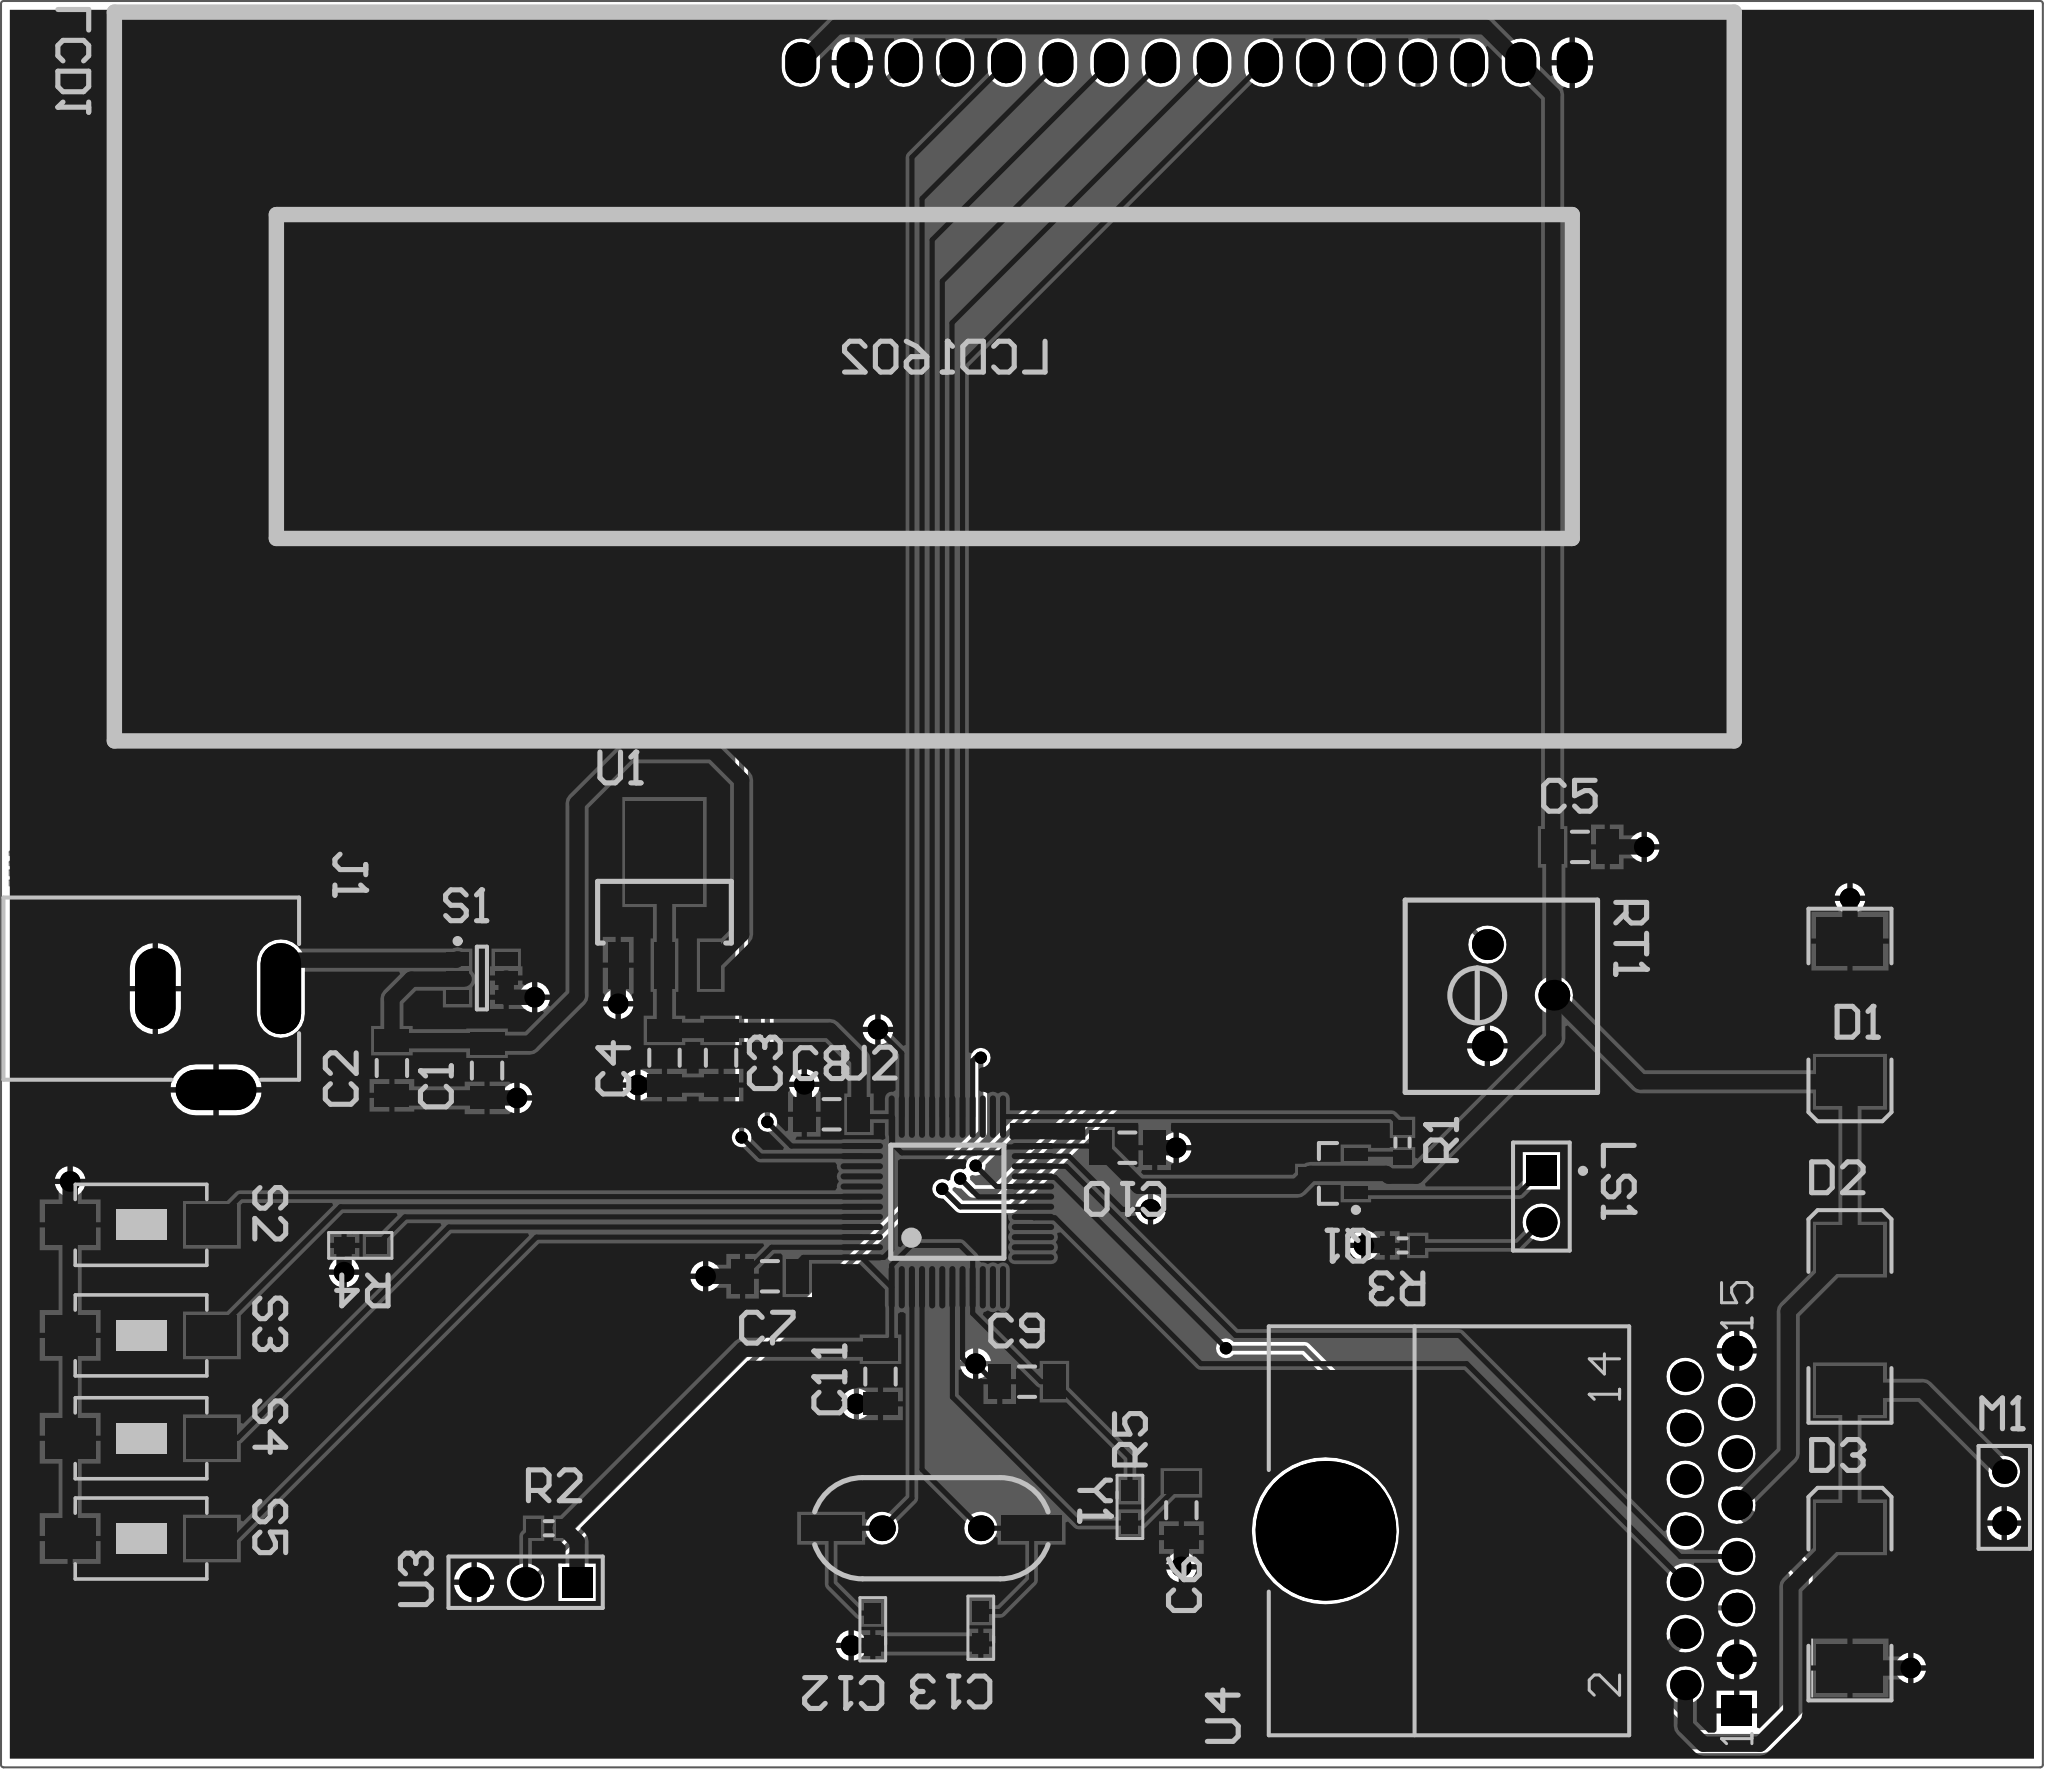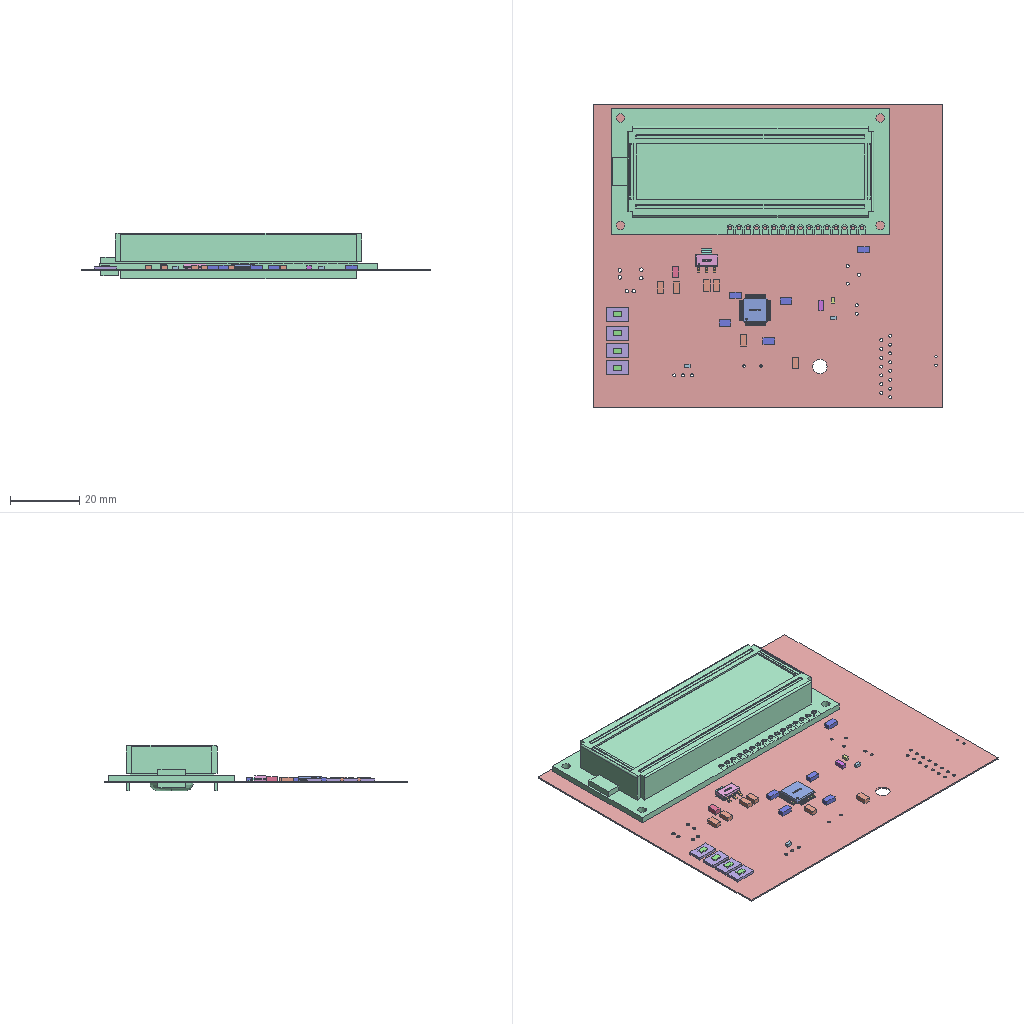Circuit board layout | Altium Designer | box 100.8 x 87.2 x 13.2 mm
Layer stack:
# Altium Designer layer stack of  (unit mm; dielectric type: 0 none, 1 core, 2 prepreg, 3 surface material)
index,name,kind,layer,copper_thickness_mm,dielectric_type,dielectric_thickness_mm,dielectric_material,dielectric_constant
0,Top Paste,other,,,,,,
1,Top Overlay,other,,,,,,
2,Top Solder,dielectric,,,3,0.0102,Solder Resist,3.5
3,Top Layer,copper,Top Layer,0.0356,,,,
4,Dielectric 1,dielectric,,,0,0.32,FR-4,4.8
5,Bottom Layer,copper,Bottom Layer,0.0356,,,,
6,Bottom Solder,dielectric,,,3,0.0102,Solder Resist,3.5
7,Bottom Overlay,other,,,,,,
8,Bottom Paste,other,,,,,,
# drill layer pairs: low layer,high layer
drill_pair,Top Layer,Bottom Layer
Part placement:
Designator,Comment,Layer,Footprint,Center-X(mm),Center-Y(mm),Rotation
Y1,12M,TopLayer,XTAL_US,72.236,37.084,360
U4,L298N,TopLayer,Multiwatt15H,101.854,36.957,90
U3,DS18B20,TopLayer,HDR1X3,52.197,34.417,180
U2,STM32F103C8T6,TopLayer,LQFP48_7X7,73.025,53.2,360
U1,AMS1117,TopLayer,SOT223,59.055,67.691,360
S5,SW-PB,TopLayer,SW_PB2_A1,33.203,36.576,270
S4,SW-PB,TopLayer,SW_PB2_A1,33.203,41.529,270
S3,SW-PB,TopLayer,SW_PB2_A1,33.203,46.609,270
S2,SW-PB,TopLayer,SW_PB2_A1,33.203,52.07,270
S1,SW DPDT,TopLayer,SOT23-6_N,50.038,64.262,360
RT1,10K,TopLayer,电位器,101.336,63.413,270
R5,Res2,TopLayer,my0603,82.042,38.138,90
R4,Res2,TopLayer,my0603,44.031,51.054,180
R3,100,TopLayer,J1-0603,95.504,51.054,180
R2,10K,TopLayer,J1-0603,53.34,37.084,0
R1,100,TopLayer,J1-0603,95.504,56.134,90
Q1,PNP,TopLayer,SOT-23B_N,92.075,54.61,180
M1,Meter,TopLayer,RAD-0.1,125.222,38.608,90
LS1,Speaker,TopLayer,PIN2,102.362,53.467,270
LCD1,LCD1602,TopLayer,LCD1602,84.836,109.474,180
J1,PWR2.5,TopLayer,KLD-0202,37.009,61.863,360
D3,Diode,TopLayer,SMC,117.602,33.655,90
D2,Diode,TopLayer,SMC,117.602,47.371,90
D1,Diode,TopLayer,SMC,117.602,62.611,270
C13,22P,TopLayer,my0603,74.676,32.169,270
C12,22P,TopLayer,my0603,69.342,32.093,270
C11,0.1UF,TopLayer,C1206,69.723,44.577,90
C10,0.1UF,TopLayer,C1206,81.915,55.88,180
C9,0.1UF,TopLayer,C1206,76.962,44.323,360
C8,0.1UF,TopLayer,C1206,67.31,57.531,360
C7,0.1UF,TopLayer,C1206,64.262,49.53,360
C6,0.1UF,TopLayer,C1206,84.582,37.973,90
C5,1U,TopLayer,C1206,104.267,70.739,0
C4,100PF,TopLayer,C1206,59.055,60.325,90
C3,100PF,TopLayer,C1206,61.849,60.325,90
C2,100PF,TopLayer,C1206,45.593,59.817,90
C1,100PF,TopLayer,C1206,50.292,59.69,90
Pad and via stacks:
# Altium Designer via and pad stacks of  (unit mm). Each distinct definition once, with the count of objects using it.
# via: kind,start_layer,end_layer,hole_mm,diameter_mm,mode(0 simple;1 top-mid-bottom;2 full stack),diameter_per_layer,count,example_net
# pad: kind,layer,hole_mm,hole_type(0 round;1 square;2 slot),plating,top_size,top_shape(1 round;2 rect;3 octagon;9 rounded rect),mid_size,bottom_size,mode,footprint,size_per_layer,count,example
pad,Top Layer,0,0,plated,1.016x2.286,2,1.016x2.286,1.016x2.286,0,SOT223,,3,U1.3
pad,Top Layer,0,0,plated,3.81x5.08,2,3.81x5.08,3.81x5.08,0,SOT223,,1,U1.2
pad,Top Layer,0,0,plated,0.65x1.1,2,0.65x1.1,0.65x1.1,0,SOT23-6_N,,6,S1.1
pad,Top Layer,0,0,plated,1.7x1.1,2,1.7x1.1,1.7x1.1,0,C1206,,22,C4.2
pad,Top Layer,0,0,plated,0.3x2.1,1,0.3x2.1,0.3x2.1,0,LQFP48 7X7,,48,U2.48
pad,Top Layer,0,0,plated,0.9x0.7,2,0.9x0.7,0.9x0.7,0,J1-0603,,6,R1.1
pad,Top Layer,0,0,plated,0.6x1.15,2,0.6x1.15,0.6x1.15,0,SOT-23B_N,,3,Q1.1
pad,Top Layer,0,0,plated,2.5x2,2,2.5x2,2.5x2,0,SW_PB2_A1,,8,S2.1
pad,Top Layer,0,0,plated,1x0.8,2,1x0.8,1x0.8,0,my0603,,8,R4.1
pad,Top Layer,0,0,plated,2.4x3.3,2,2.4x3.3,2.4x3.3,0,SMC,,6,D1.1
pad,Top Layer,0,0,plated,3x1.27,2,3x1.27,3x1.27,0,XTAL_US,,2,Y1.2
pad,Multi-Layer,0.9,0,plated,1.524x2.032,1,1.524x2.032,1.524x2.032,0,LCD1602,,16,LCD1.1
pad,Multi-Layer,0,0,plated,2x4.5,1,2x4.5,2x4.5,0,KLD-0202,,1,J1.1
pad,Multi-Layer,0,0,plated,2x4,1,2x4,2x4,0,KLD-0202,,1,J1.2
pad,Multi-Layer,0,0,plated,4x2,1,4x2,4x2,0,KLD-0202,,1,J1.3
pad,Multi-Layer,1,0,plated,1.5x1.5,1,1.5x1.5,1.5x1.5,0,KLD-0202,,6,J1.1B
pad,Multi-Layer,0.9,0,plated,1.524x1.524,1,1.524x1.524,1.524x1.524,0,\u00B5\u00E7\u00CE\u00BB\u00C6\u00F7,,3,RT1.2
pad,Multi-Layer,0.9,0,plated,1.5x1.5,2,1.5x1.5,1.5x1.5,0,PIN2,,1,LS1.1
pad,Multi-Layer,0.9,0,plated,1.5x1.5,1,1.5x1.5,1.5x1.5,0,PIN2,,1,LS1.2
pad,Multi-Layer,0.9,0,plated,1.5x1.5,2,1.5x1.5,1.5x1.5,0,HDR1X3,,1,U3.1
pad,Multi-Layer,0.9,0,plated,1.5x1.5,1,1.5x1.5,1.5x1.5,0,HDR1X3,,2,U3.2
pad,Multi-Layer,0.9,0,plated,1.5x1.5,2,1.5x1.5,1.5x1.5,0,Multiwatt15H,,1,U4.1
pad,Multi-Layer,0.9,0,plated,1.5x1.5,1,1.5x1.5,1.5x1.5,0,Multiwatt15H,,14,U4.2
pad,Multi-Layer,4.2,0,plated,6.9x6.9,1,6.9x6.9,6.9x6.9,0,Multiwatt15H,,1,U4.16
pad,Multi-Layer,0.7,0,plated,1.2x1.2,1,1.2x1.2,1.2x1.2,0,RAD-0.1,,2,M1.1
pad,Multi-Layer,0.7112,0,plated,1.27x1.27,1,1.27x1.27,1.27x1.27,0,XTAL_US,,2,Y1.2
via,Top Layer,Bottom Layer,0.508,1.016,0,,19,GND
via,Top Layer,Bottom Layer,0.3048,0.6096,0,,7,PB15
Copper pours:
name,layer,net,type(0 solid;1 hatched;2 none)
G,Top Layer,GND,0
G,Bottom Layer,GND,0
Design rules, without the lines most boards share:
# Altium Designer design rules of  (exported by Altium Designer, unit mm)
# columns: name | kind | enabled | priority | scope1 | scope2 | descriptor | typed fields (field=value)
SilkToSilkClearance | 55 | enabled | 1 | All | All | Silk to Silk (Clearance=0mil) (All),(All) |
SilkToSolderMaskClearance | 54 | enabled | 1 | IsPad | All | Silk To Solder Mask (Clearance=0mil) (IsPad),(All) |
MinimumSolderMaskSliver | 53 | enabled | 1 | All | All | Minimum Solder Mask Sliver (Gap=0mil) (All),(All) |
HoleToHoleClearance | 52 | enabled | 1 | All | All | Hole To Hole Clearance (Gap=10mil) (All),(All) | gap=0.254
DiffPairsRouting | 51 | enabled | 1 | All | All | Differential Pairs Uncoupled Length using the Gap Constraints (Min=10mil) (Max=10mil) (Prefered=10mil)  and Width Constraints (Min=15mil) (Max=15mil) (Prefered=15mil) (All) |
SolderMaskExpansion | 13 | enabled | 1 | All | All | Solder Mask Expansion (Expansion =4mil) (All) | expansion=0.1016
PasteMaskExpansion | 14 | enabled | 1 | All | All | Paste Mask Expansion (Expansion =0mil) (All) | expansion=0
RoutingVias | 11 | enabled | 1 | All | All | Routing Via (MinHoleWidth=28mil) (MaxHoleWidth=28mil) (PreferredHoleWidth=28mil) (MinWidth=50mil) (MaxWidth=50mil) (PreferedWidth=50mil) (All) | via_min_hole=0.7112 via_max_hole=0.7112 via_preferred_diameter=1.27 via_preferred_hole=0.7112
Width | 2 | enabled | 1 | All | All | Width Constraint (Min=10mil) (Max=30mil) (Preferred=10mil) (All) |
PolygonConnect | 20 | enabled | 1 | All | All | Polygon Connect Rule(Relief Connect )(Conductor Width=10mil) (Relief Angle=90 Angle) (Entries=4) (Air Gap Width=10mil) (All),(All) | connect_style(0=relief,1=direct,2=none)=0 relief_conductor_width=0.254 relief_entries=4
PlaneConnect | 6 | enabled | 1 | All | All | Power Plane Connect Rule(Relief Connect )(Expansion=20mil) (Conductor Width=10mil) (Air Gap=10mil) (Entries=4) (All) | relief_conductor_width=0.254 relief_entries=4 relief_expansion=0.508
Clearance | 0 | enabled | 1 | All | All | Clearance Constraint (Gap=7mil) (All),(All) | gap=0.1778
Classes set for this board:
# Altium Designer classes of  (member kind: 0 net, 1 component, 2 from-to, 3 pad, 4 layer, 5 differential pair, 6 design channel, 7 polygon, 8 structure, 9 xSignal)
# columns: class name | member kind | superclass | members
Sheet1 | 1 | no | C1; C2; C3; C4; C5; C6; C7; C8; C9; C10; C11; C12; C13; D1; D2; D3; J1; LCD1; LS1; M1; Q1; R1; R2; R3; R4; R5; RT1; S1; S2; S3; S4; S5; U1; U2; U3; U4; Y1;